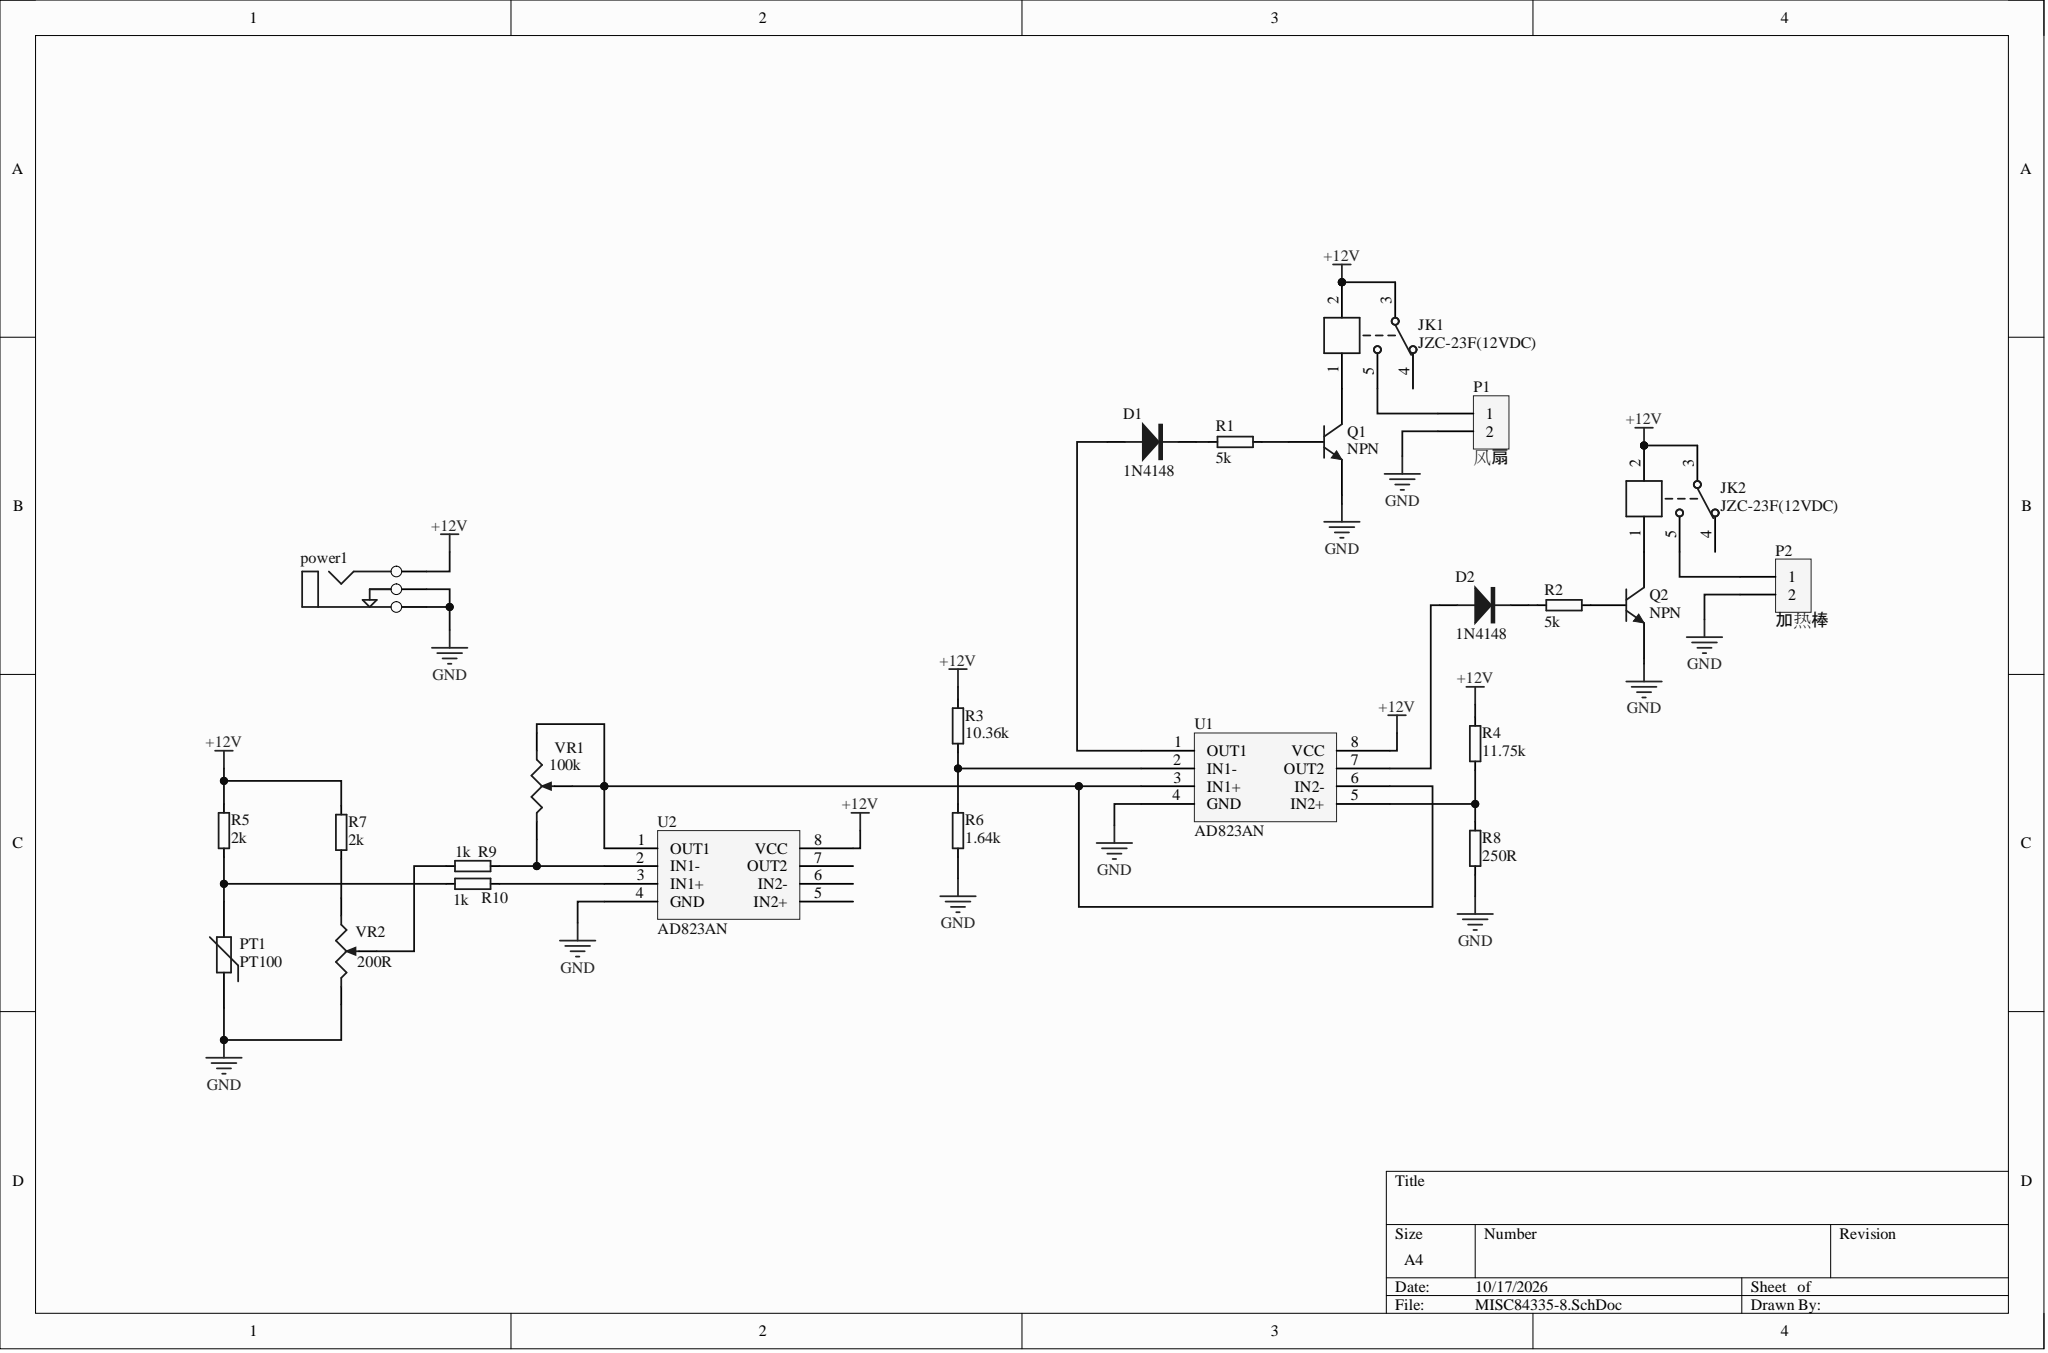Circuit board | Altium Designer | 24 parts | 20 nets
Bill of materials:
Comment,Description,Designator,Footprint,LibRef,Quantity
"1N4148","Diode","D1, D2","DO-35","DIO","2"
"JZC-23F(12VDC)","","JK1, JK2","JZC-23F(4123)","JZC-23F(5VDC)","2"
"风扇","","P1","HDR1X2","CON2","1"
"加热棒","","P2","HDR1X2","CON2","1"
"","","power1","DC-005","power2","1"
"PT100","","PT1","VDR 9D-4.5","Res Varistor","1"
"NPN","NPN Bipolar Transistor","Q1, Q2","TO-226-AA","NPN","2"
"5k","","R1, R2","RS 1/4W","RES","2"
"10.36k","","R3","RS 1/4W","RES","1"
"11.75k","","R4","RS 1/4W","RES","1"
"2k","","R5, R7","RS 1/4W","RES","2"
"1.64k","","R6","RS 1/4W","RES","1"
"250R","","R8","RS 1/4W","RES","1"
"1k","","R9, R10","RS 1/4W","RES","2"
"AD823AN","","U1, U2","DIP-8","LM358_2","2"
"100k","Potentiometer","VR1","3296W","RES-V","1"
"200R","Potentiometer","VR2","3296W","RES-V","1"
Netlist (Protel format):
[
D1
DO-35
1N4148



]
[
D2
DO-35
1N4148



]
[
JK1
JZC-23F(4123)
JZC-23F(12VDC)



]
[
JK2
JZC-23F(4123)
JZC-23F(12VDC)



]
[
P1
HDR1X2
风扇



]
[
P2
HDR1X2
加热棒



]
[
power1
DC-005




]
[
PT1
VDR 9D-4.5
PT100



]
[
Q1
TO-226-AA
NPN



]
[
Q2
TO-226-AA
NPN



]
[
R1
RS 1/4W
5k



]
[
R2
RS 1/4W
5k



]
[
R3
RS 1/4W
10.36k



]
[
R4
RS 1/4W
11.75k



]
[
R5
RS 1/4W
2k



]
[
R6
RS 1/4W
1.64k



]
[
R7
RS 1/4W
2k



]
[
R8
RS 1/4W
250R



]
[
R9
RS 1/4W
1k



]
[
R10
RS 1/4W
1k



]
[
U1
DIP-8
AD823AN



]
[
U2
DIP-8
AD823AN



]
[
VR1
3296W
100k



]
[
VR2
3296W
200R



]
(
NetU1_3
U1-3
U1-6
U2-1
VR1-1
VR1-2
)
(
NetR10_1
R10-1
U2-3
)
(
NetR9_2
R9-2
VR2-2
)
(
NetR9_1
R9-1
U2-2
VR1-3
)
(
NetR7_1
R7-1
VR2-1
)
(
NetR4_1
R4-1
R8-2
U1-5
)
(
NetR3_1
R3-1
R6-2
U1-2
)
(
NetQ2_2
Q2-2
R2-1
)
(
NetQ1_2
Q1-2
R1-1
)
(
NetPT1_2
PT1-2
R5-1
R10-2
)
(
NetJK2_5
JK2-5
P2-1
)
(
NetJK2_1
JK2-1
Q2-1
)
(
NetJK1_5
JK1-5
P1-1
)
(
NetJK1_1
JK1-1
Q1-1
)
(
NetD2_2
D2-2
R2-2
)
(
NetD2_1
D2-1
U1-7
)
(
NetD1_2
D1-2
R1-2
)
(
NetD1_1
D1-1
U1-1
)
(
GND
P1-2
P2-2
power1-2
power1-3
PT1-1
Q1-3
Q2-3
R6-1
R8-1
U1-4
U2-4
VR2-3
)
(
+12V
JK1-2
JK1-3
JK2-2
JK2-3
power1-1
R3-2
R4-2
R5-2
R7-2
U1-8
U2-8
)